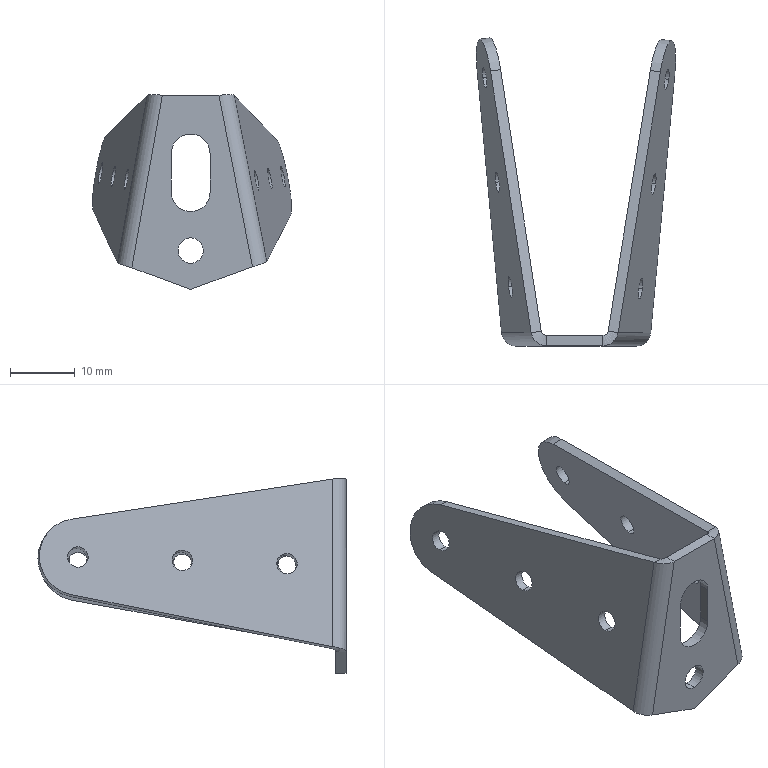Part | SolidWorks | features BaseBody 1 | 1 solid | 42 faces | box 30.783 x 47.582 x 30.086 mm | volume 3238 mm3 | cylinder 23 | plane 15 | spline 4 | commonest cylinder face diameters 3.2 x12 6 x3 1.473 x2 3.937 x2 4.673 x2 12 x2